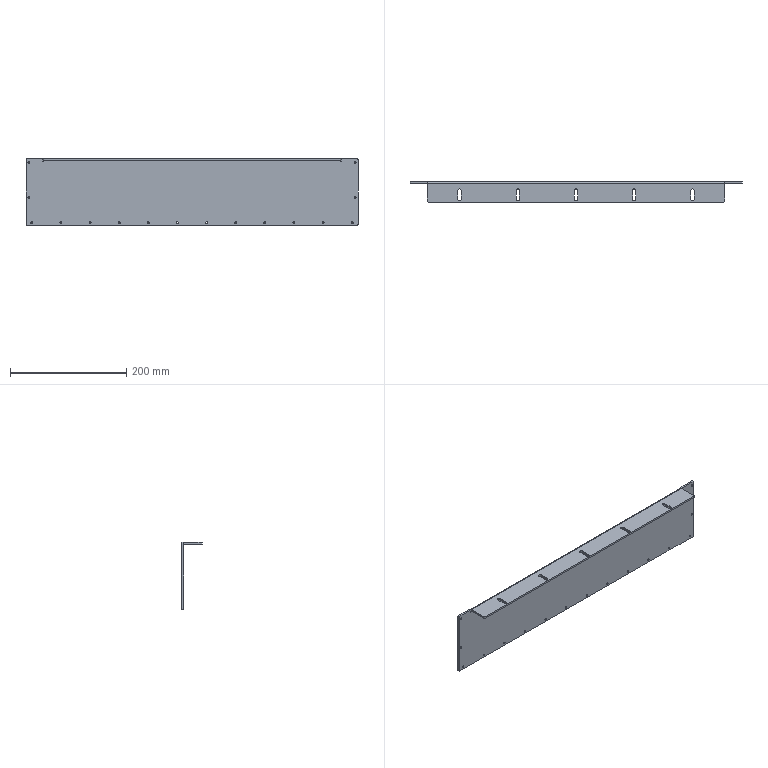Part | STEP file | 1 solid | 85 faces | box 570 x 35 x 115.5 mm | volume 243087 mm3 | cylinder 55 | plane 30 | commonest cylinder face diameters 3.3 x32 5.5 x15 4 x6 1 x1 7 x1